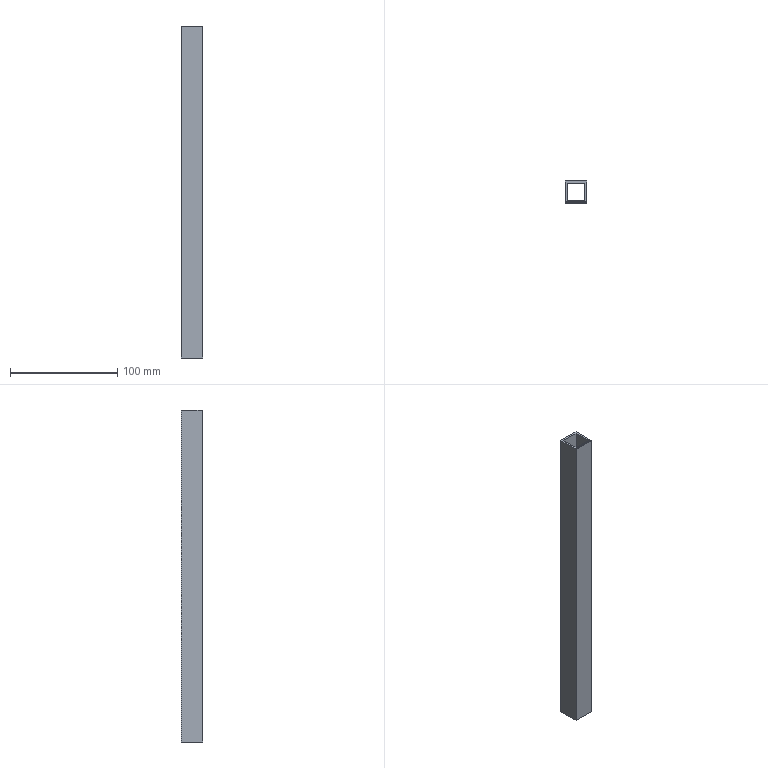Part | NX | features BREP 1 | 1 solid | 11 faces | box 20 x 20 x 309.106 mm | volume 44509 mm3 | plane 11
STEP:
#1=CARTESIAN_POINT('',(1630.423,-697.5,418.077));
#2=VERTEX_POINT('',#1);
#3=CARTESIAN_POINT('',(1610.423,-697.5,418.106));
#4=VERTEX_POINT('',#3);
#5=CARTESIAN_POINT('',(1620.423,-697.5,418.091));
#6=DIRECTION('',(-1.,0.,0.001449));
#7=VECTOR('',#6,1000.);
#8=LINE('',#5,#7);
#9=EDGE_CURVE('',#2,#4,#8,.T.);
#10=ORIENTED_EDGE('',*,*,#9,.T.);
#11=CARTESIAN_POINT('',(1610.423,-698.,418.106));
#12=VERTEX_POINT('',#11);
#13=CARTESIAN_POINT('',(1610.423,-697.5,418.106));
#14=CARTESIAN_POINT('',(1610.423,-698.,418.106));
#15=B_SPLINE_CURVE_WITH_KNOTS('',1,(#13,#14),.UNSPECIFIED.,.F.,.F.,(2,2),(19.5,20.),.UNSPECIFIED.);
#16=EDGE_CURVE('',#4,#12,#15,.T.);
#17=ORIENTED_EDGE('',*,*,#16,.T.);
#18=CARTESIAN_POINT('',(1630.423,-698.,418.077));
#19=VERTEX_POINT('',#18);
#20=CARTESIAN_POINT('',(1620.423,-698.,418.091));
#21=DIRECTION('',(-1.,0.,0.001449));
#22=VECTOR('',#21,1000.);
#23=LINE('',#20,#22);
#24=EDGE_CURVE('',#19,#12,#23,.T.);
#25=ORIENTED_EDGE('',*,*,#24,.F.);
#26=CARTESIAN_POINT('',(1630.423,-697.75,418.077));
#27=DIRECTION('',(0.,1.,0.000000007));
#28=VECTOR('',#27,1000.);
#29=LINE('',#26,#28);
#30=EDGE_CURVE('',#19,#2,#29,.T.);
#31=ORIENTED_EDGE('',*,*,#30,.T.);
#32=EDGE_LOOP('',(#10,#17,#25,#31));
#33=FACE_BOUND('',#32,.T.);
#34=CARTESIAN_POINT('',(1662.694,-697.768,418.03));
#35=DIRECTION('',(0.001449,0.,1.));
#36=DIRECTION('',(1.,0.,-0.001449));
#37=AXIS2_PLACEMENT_3D('',#34,#35,#36);
#38=PLANE('',#37);
#39=ADVANCED_FACE('',(#33),#38,.T.);
#40=CARTESIAN_POINT('',(1612.423,-680.,418.103));
#41=VERTEX_POINT('',#40);
#42=CARTESIAN_POINT('',(1628.423,-680.,418.08));
#43=VERTEX_POINT('',#42);
#44=CARTESIAN_POINT('',(1620.423,-680.,418.091));
#45=DIRECTION('',(1.,0.,-0.001449));
#46=VECTOR('',#45,1000.);
#47=LINE('',#44,#46);
#48=EDGE_CURVE('',#41,#43,#47,.T.);
#49=ORIENTED_EDGE('',*,*,#48,.T.);
#50=CARTESIAN_POINT('',(1628.423,-696.,418.08));
#51=VERTEX_POINT('',#50);
#52=CARTESIAN_POINT('',(1628.423,-688.,418.08));
#53=DIRECTION('',(0.,1.,0.));
#54=VECTOR('',#53,1000.);
#55=LINE('',#52,#54);
#56=EDGE_CURVE('',#51,#43,#55,.T.);
#57=ORIENTED_EDGE('',*,*,#56,.F.);
#58=CARTESIAN_POINT('',(1612.423,-696.,418.103));
#59=VERTEX_POINT('',#58);
#60=CARTESIAN_POINT('',(1620.423,-696.,418.091));
#61=DIRECTION('',(1.,0.,-0.001449));
#62=VECTOR('',#61,1000.);
#63=LINE('',#60,#62);
#64=EDGE_CURVE('',#59,#51,#63,.T.);
#65=ORIENTED_EDGE('',*,*,#64,.F.);
#66=CARTESIAN_POINT('',(1612.423,-688.,418.103));
#67=DIRECTION('',(0.,-1.,0.));
#68=VECTOR('',#67,1000.);
#69=LINE('',#66,#68);
#70=EDGE_CURVE('',#41,#59,#69,.T.);
#71=ORIENTED_EDGE('',*,*,#70,.F.);
#72=EDGE_LOOP('',(#49,#57,#65,#71));
#73=FACE_BOUND('',#72,.T.);
#74=ORIENTED_EDGE('',*,*,#9,.F.);
#75=CARTESIAN_POINT('',(1630.423,-678.,418.077));
#76=VERTEX_POINT('',#75);
#77=CARTESIAN_POINT('',(1630.423,-687.75,418.077));
#78=DIRECTION('',(0.,1.,0.));
#79=VECTOR('',#78,1000.);
#80=LINE('',#77,#79);
#81=EDGE_CURVE('',#2,#76,#80,.T.);
#82=ORIENTED_EDGE('',*,*,#81,.T.);
#83=CARTESIAN_POINT('',(1610.423,-678.,418.106));
#84=VERTEX_POINT('',#83);
#85=CARTESIAN_POINT('',(1620.423,-678.,418.091));
#86=DIRECTION('',(1.,0.,-0.001449));
#87=VECTOR('',#86,1000.);
#88=LINE('',#85,#87);
#89=EDGE_CURVE('',#84,#76,#88,.T.);
#90=ORIENTED_EDGE('',*,*,#89,.F.);
#91=CARTESIAN_POINT('',(1610.423,-678.,418.106));
#92=CARTESIAN_POINT('',(1610.423,-697.5,418.106));
#93=B_SPLINE_CURVE_WITH_KNOTS('',1,(#91,#92),.UNSPECIFIED.,.F.,.F.,(2,2),(0.,19.5),.UNSPECIFIED.);
#94=EDGE_CURVE('',#84,#4,#93,.T.);
#95=ORIENTED_EDGE('',*,*,#94,.T.);
#96=EDGE_LOOP('',(#74,#82,#90,#95));
#97=FACE_BOUND('',#96,.T.);
#98=CARTESIAN_POINT('',(1601.46,-661.999,418.119));
#99=DIRECTION('',(0.001449,0.,1.));
#100=DIRECTION('',(1.,0.,-0.001449));
#101=AXIS2_PLACEMENT_3D('',#98,#99,#100);
#102=PLANE('',#101);
#103=ADVANCED_FACE('',(#73,#97),#102,.T.);
#104=ORIENTED_EDGE('',*,*,#64,.T.);
#105=CARTESIAN_POINT('',(1628.423,-696.,109.));
#106=VERTEX_POINT('',#105);
#107=CARTESIAN_POINT('',(1628.423,-696.,263.54));
#108=DIRECTION('',(0.,0.,1.));
#109=VECTOR('',#108,1000.);
#110=LINE('',#107,#109);
#111=EDGE_CURVE('',#106,#51,#110,.T.);
#112=ORIENTED_EDGE('',*,*,#111,.F.);
#113=CARTESIAN_POINT('',(1612.423,-696.,109.));
#114=VERTEX_POINT('',#113);
#115=CARTESIAN_POINT('',(1620.423,-696.,109.));
#116=DIRECTION('',(1.,0.,0.));
#117=VECTOR('',#116,1000.);
#118=LINE('',#115,#117);
#119=EDGE_CURVE('',#114,#106,#118,.T.);
#120=ORIENTED_EDGE('',*,*,#119,.F.);
#121=CARTESIAN_POINT('',(1612.423,-696.,263.551));
#122=DIRECTION('',(0.,0.,1.));
#123=VECTOR('',#122,1000.);
#124=LINE('',#121,#123);
#125=EDGE_CURVE('',#114,#59,#124,.T.);
#126=ORIENTED_EDGE('',*,*,#125,.T.);
#127=EDGE_LOOP('',(#104,#112,#120,#126));
#128=FACE_BOUND('',#127,.T.);
#129=CARTESIAN_POINT('',(1630.423,-696.,-71.091));
#130=DIRECTION('',(0.,-1.,0.));
#131=DIRECTION('',(0.,0.,1.));
#132=AXIS2_PLACEMENT_3D('',#129,#130,#131);
#133=PLANE('',#132);
#134=ADVANCED_FACE('',(#128),#133,.F.);
#135=ORIENTED_EDGE('',*,*,#125,.F.);
#136=CARTESIAN_POINT('',(1612.423,-680.,109.));
#137=VERTEX_POINT('',#136);
#138=CARTESIAN_POINT('',(1612.423,-688.,109.));
#139=DIRECTION('',(0.,1.,0.));
#140=VECTOR('',#139,1000.);
#141=LINE('',#138,#140);
#142=EDGE_CURVE('',#114,#137,#141,.T.);
#143=ORIENTED_EDGE('',*,*,#142,.T.);
#144=CARTESIAN_POINT('',(1612.423,-680.,263.551));
#145=DIRECTION('',(0.,0.,1.));
#146=VECTOR('',#145,1000.);
#147=LINE('',#144,#146);
#148=EDGE_CURVE('',#137,#41,#147,.T.);
#149=ORIENTED_EDGE('',*,*,#148,.T.);
#150=ORIENTED_EDGE('',*,*,#70,.T.);
#151=EDGE_LOOP('',(#135,#143,#149,#150));
#152=FACE_BOUND('',#151,.T.);
#153=CARTESIAN_POINT('',(1612.423,-680.,109.));
#154=DIRECTION('',(1.,0.,0.));
#155=DIRECTION('',(0.,0.,1.));
#156=AXIS2_PLACEMENT_3D('',#153,#154,#155);
#157=PLANE('',#156);
#158=ADVANCED_FACE('',(#152),#157,.T.);
#159=ORIENTED_EDGE('',*,*,#148,.F.);
#160=CARTESIAN_POINT('',(1628.423,-680.,109.));
#161=VERTEX_POINT('',#160);
#162=CARTESIAN_POINT('',(1620.423,-680.,109.));
#163=DIRECTION('',(1.,0.,0.));
#164=VECTOR('',#163,1000.);
#165=LINE('',#162,#164);
#166=EDGE_CURVE('',#137,#161,#165,.T.);
#167=ORIENTED_EDGE('',*,*,#166,.T.);
#168=CARTESIAN_POINT('',(1628.423,-680.,263.54));
#169=DIRECTION('',(0.,0.,1.));
#170=VECTOR('',#169,1000.);
#171=LINE('',#168,#170);
#172=EDGE_CURVE('',#161,#43,#171,.T.);
#173=ORIENTED_EDGE('',*,*,#172,.T.);
#174=ORIENTED_EDGE('',*,*,#48,.F.);
#175=EDGE_LOOP('',(#159,#167,#173,#174));
#176=FACE_BOUND('',#175,.T.);
#177=CARTESIAN_POINT('',(1630.423,-680.,-71.091));
#178=DIRECTION('',(0.,-1.,0.));
#179=DIRECTION('',(0.,0.,1.));
#180=AXIS2_PLACEMENT_3D('',#177,#178,#179);
#181=PLANE('',#180);
#182=ADVANCED_FACE('',(#176),#181,.T.);
#183=ORIENTED_EDGE('',*,*,#172,.F.);
#184=CARTESIAN_POINT('',(1628.423,-688.,109.));
#185=DIRECTION('',(0.,1.,0.));
#186=VECTOR('',#185,1000.);
#187=LINE('',#184,#186);
#188=EDGE_CURVE('',#106,#161,#187,.T.);
#189=ORIENTED_EDGE('',*,*,#188,.F.);
#190=ORIENTED_EDGE('',*,*,#111,.T.);
#191=ORIENTED_EDGE('',*,*,#56,.T.);
#192=EDGE_LOOP('',(#183,#189,#190,#191));
#193=FACE_BOUND('',#192,.T.);
#194=CARTESIAN_POINT('',(1628.423,-698.,78.909));
#195=DIRECTION('',(-1.,0.,0.));
#196=DIRECTION('',(0.,0.,1.));
#197=AXIS2_PLACEMENT_3D('',#194,#195,#196);
#198=PLANE('',#197);
#199=ADVANCED_FACE('',(#193),#198,.T.);
#200=ORIENTED_EDGE('',*,*,#16,.F.);
#201=ORIENTED_EDGE('',*,*,#94,.F.);
#202=CARTESIAN_POINT('',(1610.423,-678.,109.));
#203=VERTEX_POINT('',#202);
#204=CARTESIAN_POINT('',(1610.423,-678.,263.553));
#205=DIRECTION('',(0.,0.,1.));
#206=VECTOR('',#205,1000.);
#207=LINE('',#204,#206);
#208=EDGE_CURVE('',#203,#84,#207,.T.);
#209=ORIENTED_EDGE('',*,*,#208,.F.);
#210=CARTESIAN_POINT('',(1610.423,-698.,109.));
#211=VERTEX_POINT('',#210);
#212=CARTESIAN_POINT('',(1610.423,-688.,109.));
#213=DIRECTION('',(0.,1.,0.));
#214=VECTOR('',#213,1000.);
#215=LINE('',#212,#214);
#216=EDGE_CURVE('',#211,#203,#215,.T.);
#217=ORIENTED_EDGE('',*,*,#216,.F.);
#218=CARTESIAN_POINT('',(1610.423,-698.,263.553));
#219=DIRECTION('',(0.,0.,-1.));
#220=VECTOR('',#219,1000.);
#221=LINE('',#218,#220);
#222=EDGE_CURVE('',#12,#211,#221,.T.);
#223=ORIENTED_EDGE('',*,*,#222,.F.);
#224=EDGE_LOOP('',(#200,#201,#209,#217,#223));
#225=FACE_BOUND('',#224,.T.);
#226=CARTESIAN_POINT('',(1610.423,-688.,675.409));
#227=DIRECTION('',(1.,0.,0.));
#228=DIRECTION('',(0.,1.,0.));
#229=AXIS2_PLACEMENT_3D('',#226,#227,#228);
#230=PLANE('',#229);
#231=ADVANCED_FACE('',(#225),#230,.F.);
#232=ORIENTED_EDGE('',*,*,#222,.T.);
#233=CARTESIAN_POINT('',(1630.423,-698.,109.));
#234=VERTEX_POINT('',#233);
#235=CARTESIAN_POINT('',(1620.423,-698.,109.));
#236=DIRECTION('',(1.,0.,0.));
#237=VECTOR('',#236,1000.);
#238=LINE('',#235,#237);
#239=EDGE_CURVE('',#211,#234,#238,.T.);
#240=ORIENTED_EDGE('',*,*,#239,.T.);
#241=CARTESIAN_POINT('',(1630.423,-698.,263.538));
#242=DIRECTION('',(0.,0.,1.));
#243=VECTOR('',#242,1000.);
#244=LINE('',#241,#243);
#245=EDGE_CURVE('',#234,#19,#244,.T.);
#246=ORIENTED_EDGE('',*,*,#245,.T.);
#247=ORIENTED_EDGE('',*,*,#24,.T.);
#248=EDGE_LOOP('',(#232,#240,#246,#247));
#249=FACE_BOUND('',#248,.T.);
#250=CARTESIAN_POINT('',(1630.423,-698.,-71.091));
#251=DIRECTION('',(0.,-1.,0.));
#252=DIRECTION('',(0.,0.,1.));
#253=AXIS2_PLACEMENT_3D('',#250,#251,#252);
#254=PLANE('',#253);
#255=ADVANCED_FACE('',(#249),#254,.T.);
#256=ORIENTED_EDGE('',*,*,#81,.F.);
#257=ORIENTED_EDGE('',*,*,#30,.F.);
#258=ORIENTED_EDGE('',*,*,#245,.F.);
#259=CARTESIAN_POINT('',(1630.423,-678.,109.));
#260=VERTEX_POINT('',#259);
#261=CARTESIAN_POINT('',(1630.423,-688.,109.));
#262=DIRECTION('',(0.,1.,0.));
#263=VECTOR('',#262,1000.);
#264=LINE('',#261,#263);
#265=EDGE_CURVE('',#234,#260,#264,.T.);
#266=ORIENTED_EDGE('',*,*,#265,.T.);
#267=CARTESIAN_POINT('',(1630.423,-678.,263.538));
#268=DIRECTION('',(0.,0.,1.));
#269=VECTOR('',#268,1000.);
#270=LINE('',#267,#269);
#271=EDGE_CURVE('',#260,#76,#270,.T.);
#272=ORIENTED_EDGE('',*,*,#271,.T.);
#273=EDGE_LOOP('',(#256,#257,#258,#266,#272));
#274=FACE_BOUND('',#273,.T.);
#275=CARTESIAN_POINT('',(1630.423,-698.,78.909));
#276=DIRECTION('',(-1.,0.,0.));
#277=DIRECTION('',(0.,0.,1.));
#278=AXIS2_PLACEMENT_3D('',#275,#276,#277);
#279=PLANE('',#278);
#280=ADVANCED_FACE('',(#274),#279,.F.);
#281=ORIENTED_EDGE('',*,*,#89,.T.);
#282=ORIENTED_EDGE('',*,*,#271,.F.);
#283=CARTESIAN_POINT('',(1620.423,-678.,109.));
#284=DIRECTION('',(1.,0.,0.));
#285=VECTOR('',#284,1000.);
#286=LINE('',#283,#285);
#287=EDGE_CURVE('',#203,#260,#286,.T.);
#288=ORIENTED_EDGE('',*,*,#287,.F.);
#289=ORIENTED_EDGE('',*,*,#208,.T.);
#290=EDGE_LOOP('',(#281,#282,#288,#289));
#291=FACE_BOUND('',#290,.T.);
#292=CARTESIAN_POINT('',(1630.423,-678.,-71.091));
#293=DIRECTION('',(0.,-1.,0.));
#294=DIRECTION('',(0.,0.,1.));
#295=AXIS2_PLACEMENT_3D('',#292,#293,#294);
#296=PLANE('',#295);
#297=ADVANCED_FACE('',(#291),#296,.F.);
#298=ORIENTED_EDGE('',*,*,#188,.T.);
#299=ORIENTED_EDGE('',*,*,#166,.F.);
#300=ORIENTED_EDGE('',*,*,#142,.F.);
#301=ORIENTED_EDGE('',*,*,#119,.T.);
#302=EDGE_LOOP('',(#298,#299,#300,#301));
#303=FACE_BOUND('',#302,.T.);
#304=ORIENTED_EDGE('',*,*,#287,.T.);
#305=ORIENTED_EDGE('',*,*,#265,.F.);
#306=ORIENTED_EDGE('',*,*,#239,.F.);
#307=ORIENTED_EDGE('',*,*,#216,.T.);
#308=EDGE_LOOP('',(#304,#305,#306,#307));
#309=FACE_BOUND('',#308,.T.);
#310=CARTESIAN_POINT('',(689.366,-698.,109.));
#311=DIRECTION('',(0.,0.,1.));
#312=DIRECTION('',(1.,0.,0.));
#313=AXIS2_PLACEMENT_3D('',#310,#311,#312);
#314=PLANE('',#313);
#315=ADVANCED_FACE('',(#303,#309),#314,.F.);
#316=CLOSED_SHELL('',(#39,#103,#134,#158,#182,#199,#231,#255,#280,#297,#315));
#317=MANIFOLD_SOLID_BREP('',#316);
#318=(LENGTH_UNIT()NAMED_UNIT(*)SI_UNIT(.MILLI.,.METRE.));
#319=UNCERTAINTY_MEASURE_WITH_UNIT(LENGTH_MEASURE(0.00001),#318,'','');
#320=(NAMED_UNIT(*)PLANE_ANGLE_UNIT()SI_UNIT($,.RADIAN.));
#321=(NAMED_UNIT(*)SI_UNIT($,.STERADIAN.)SOLID_ANGLE_UNIT());
#322=(GEOMETRIC_REPRESENTATION_CONTEXT(3)GLOBAL_UNCERTAINTY_ASSIGNED_CONTEXT((#319))GLOBAL_UNIT_ASSIGNED_CONTEXT((#318,#320,#321))REPRESENTATION_CONTEXT('',''));
#323=ADVANCED_BREP_SHAPE_REPRESENTATION('',(#317),#322);